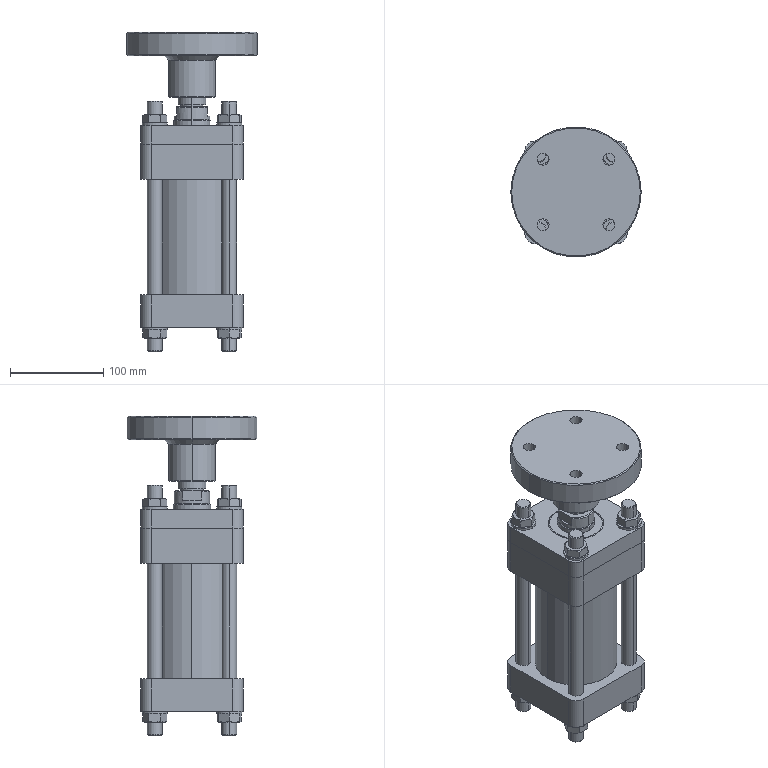Part | SolidWorks | 8 solids | 320 faces | box 140 x 140 x 343.064 mm | volume 2413914 mm3 | plane 115 | cylinder 112 | cone 91 | torus 2 | commonest cylinder face diameters 16 x48 26.88 x16 22 x12 13 x8 40 x6 19.793 x4